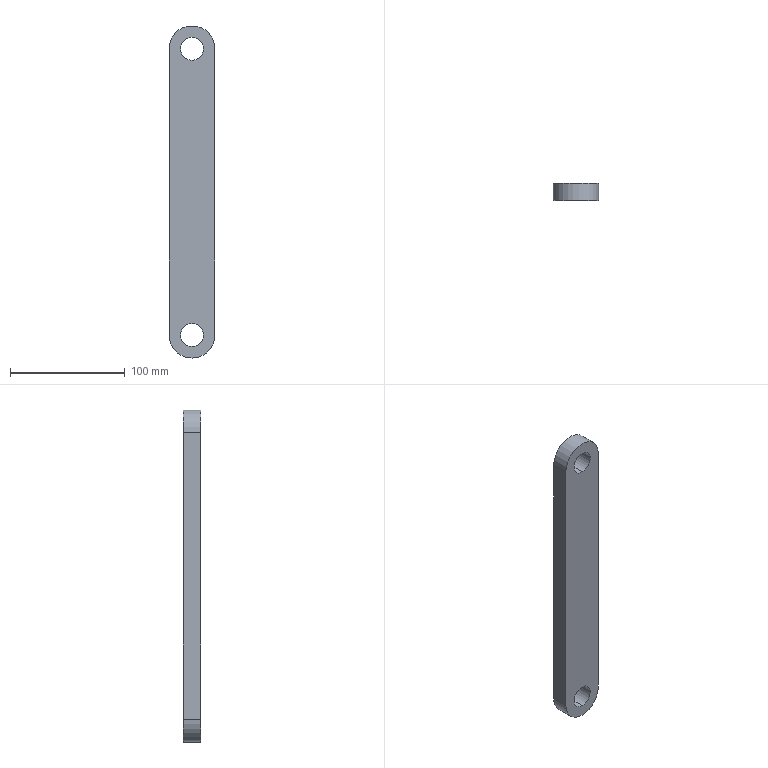Part | SolidWorks | features Extrusion 1 | 1 solid | 11 faces | box 40 x 15 x 290 mm | volume 159425 mm3 | cylinder 7 | plane 4 | commonest cylinder face diameters 20 x4 40 x3
STEP:
#1=CARTESIAN_POINT('',(0.,15.,-10.));
#2=VERTEX_POINT('',#1);
#3=CARTESIAN_POINT('',(0.,15.,10.));
#4=VERTEX_POINT('',#3);
#5=CARTESIAN_POINT('',(0.,15.,0.));
#6=DIRECTION('',(0.,1.,0.));
#7=DIRECTION('',(0.,0.,1.));
#8=AXIS2_PLACEMENT_3D('',#5,#6,#7);
#9=CIRCLE('',#8,10.);
#10=EDGE_CURVE('',#2,#4,#9,.T.);
#11=ORIENTED_EDGE('',*,*,#10,.T.);
#12=CARTESIAN_POINT('',(0.,0.,10.));
#13=VERTEX_POINT('',#12);
#14=CARTESIAN_POINT('',(0.,15.,10.));
#15=DIRECTION('',(0.,-1.,0.));
#16=VECTOR('',#15,1000.);
#17=LINE('',#14,#16);
#18=EDGE_CURVE('',#4,#13,#17,.T.);
#19=ORIENTED_EDGE('',*,*,#18,.T.);
#20=CARTESIAN_POINT('',(0.,0.,-10.));
#21=VERTEX_POINT('',#20);
#22=CARTESIAN_POINT('',(0.,0.,0.));
#23=DIRECTION('',(0.,1.,0.));
#24=DIRECTION('',(0.,0.,1.));
#25=AXIS2_PLACEMENT_3D('',#22,#23,#24);
#26=CIRCLE('',#25,10.);
#27=EDGE_CURVE('',#21,#13,#26,.T.);
#28=ORIENTED_EDGE('',*,*,#27,.F.);
#29=CARTESIAN_POINT('',(0.,15.,-10.));
#30=DIRECTION('',(0.,-1.,0.));
#31=VECTOR('',#30,1000.);
#32=LINE('',#29,#31);
#33=EDGE_CURVE('',#2,#21,#32,.T.);
#34=ORIENTED_EDGE('',*,*,#33,.F.);
#35=EDGE_LOOP('',(#11,#19,#28,#34));
#36=FACE_OUTER_BOUND('',#35,.T.);
#37=CARTESIAN_POINT('',(0.,15.,0.));
#38=DIRECTION('',(0.,-1.,0.));
#39=DIRECTION('',(0.,0.,-1.));
#40=AXIS2_PLACEMENT_3D('',#37,#38,#39);
#41=CYLINDRICAL_SURFACE('',#40,10.);
#42=ADVANCED_FACE('',(#36),#41,.F.);
#43=CARTESIAN_POINT('',(0.,15.,-260.));
#44=VERTEX_POINT('',#43);
#45=CARTESIAN_POINT('',(0.,15.,-240.));
#46=VERTEX_POINT('',#45);
#47=CARTESIAN_POINT('',(0.,15.,-250.));
#48=DIRECTION('',(0.,1.,0.));
#49=DIRECTION('',(0.,0.,1.));
#50=AXIS2_PLACEMENT_3D('',#47,#48,#49);
#51=CIRCLE('',#50,10.);
#52=EDGE_CURVE('',#44,#46,#51,.T.);
#53=ORIENTED_EDGE('',*,*,#52,.T.);
#54=CARTESIAN_POINT('',(0.,0.,-240.));
#55=VERTEX_POINT('',#54);
#56=CARTESIAN_POINT('',(0.,15.,-240.));
#57=DIRECTION('',(0.,-1.,0.));
#58=VECTOR('',#57,1000.);
#59=LINE('',#56,#58);
#60=EDGE_CURVE('',#46,#55,#59,.T.);
#61=ORIENTED_EDGE('',*,*,#60,.T.);
#62=CARTESIAN_POINT('',(0.,0.,-260.));
#63=VERTEX_POINT('',#62);
#64=CARTESIAN_POINT('',(0.,0.,-250.));
#65=DIRECTION('',(0.,1.,0.));
#66=DIRECTION('',(0.,0.,1.));
#67=AXIS2_PLACEMENT_3D('',#64,#65,#66);
#68=CIRCLE('',#67,10.);
#69=EDGE_CURVE('',#63,#55,#68,.T.);
#70=ORIENTED_EDGE('',*,*,#69,.F.);
#71=CARTESIAN_POINT('',(0.,15.,-260.));
#72=DIRECTION('',(0.,-1.,0.));
#73=VECTOR('',#72,1000.);
#74=LINE('',#71,#73);
#75=EDGE_CURVE('',#44,#63,#74,.T.);
#76=ORIENTED_EDGE('',*,*,#75,.F.);
#77=EDGE_LOOP('',(#53,#61,#70,#76));
#78=FACE_OUTER_BOUND('',#77,.T.);
#79=CARTESIAN_POINT('',(0.,15.,-250.));
#80=DIRECTION('',(0.,-1.,0.));
#81=DIRECTION('',(0.,0.,-1.));
#82=AXIS2_PLACEMENT_3D('',#79,#80,#81);
#83=CYLINDRICAL_SURFACE('',#82,10.);
#84=ADVANCED_FACE('',(#78),#83,.F.);
#85=CARTESIAN_POINT('',(0.,15.,-270.));
#86=VERTEX_POINT('',#85);
#87=CARTESIAN_POINT('',(-20.,15.,-250.));
#88=VERTEX_POINT('',#87);
#89=CARTESIAN_POINT('',(0.,15.,-250.));
#90=DIRECTION('',(0.,1.,0.));
#91=DIRECTION('',(0.,0.,1.));
#92=AXIS2_PLACEMENT_3D('',#89,#90,#91);
#93=CIRCLE('',#92,20.);
#94=EDGE_CURVE('',#86,#88,#93,.T.);
#95=ORIENTED_EDGE('',*,*,#94,.F.);
#96=CARTESIAN_POINT('',(0.,0.,-270.));
#97=VERTEX_POINT('',#96);
#98=CARTESIAN_POINT('',(0.,15.,-270.));
#99=DIRECTION('',(0.,-1.,0.));
#100=VECTOR('',#99,1000.);
#101=LINE('',#98,#100);
#102=EDGE_CURVE('',#86,#97,#101,.T.);
#103=ORIENTED_EDGE('',*,*,#102,.T.);
#104=CARTESIAN_POINT('',(-20.,0.,-250.));
#105=VERTEX_POINT('',#104);
#106=CARTESIAN_POINT('',(0.,0.,-250.));
#107=DIRECTION('',(0.,1.,0.));
#108=DIRECTION('',(0.,0.,1.));
#109=AXIS2_PLACEMENT_3D('',#106,#107,#108);
#110=CIRCLE('',#109,20.);
#111=EDGE_CURVE('',#97,#105,#110,.T.);
#112=ORIENTED_EDGE('',*,*,#111,.T.);
#113=CARTESIAN_POINT('',(-20.,15.,-250.));
#114=DIRECTION('',(0.,-1.,0.));
#115=VECTOR('',#114,1000.);
#116=LINE('',#113,#115);
#117=EDGE_CURVE('',#88,#105,#116,.T.);
#118=ORIENTED_EDGE('',*,*,#117,.F.);
#119=EDGE_LOOP('',(#95,#103,#112,#118));
#120=FACE_OUTER_BOUND('',#119,.T.);
#121=CARTESIAN_POINT('',(0.,15.,-250.));
#122=DIRECTION('',(0.,-1.,0.));
#123=DIRECTION('',(0.,0.,-1.));
#124=AXIS2_PLACEMENT_3D('',#121,#122,#123);
#125=CYLINDRICAL_SURFACE('',#124,20.);
#126=ADVANCED_FACE('',(#120),#125,.T.);
#127=ORIENTED_EDGE('',*,*,#52,.F.);
#128=CARTESIAN_POINT('',(0.,15.,-250.));
#129=DIRECTION('',(0.,1.,0.));
#130=DIRECTION('',(0.,0.,1.));
#131=AXIS2_PLACEMENT_3D('',#128,#129,#130);
#132=CIRCLE('',#131,10.);
#133=EDGE_CURVE('',#46,#44,#132,.T.);
#134=ORIENTED_EDGE('',*,*,#133,.F.);
#135=EDGE_LOOP('',(#127,#134));
#136=FACE_BOUND('',#135,.T.);
#137=CARTESIAN_POINT('',(-20.,15.,0.));
#138=VERTEX_POINT('',#137);
#139=CARTESIAN_POINT('',(20.,15.,0.));
#140=VERTEX_POINT('',#139);
#141=CARTESIAN_POINT('',(0.,15.,0.));
#142=DIRECTION('',(0.,1.,0.));
#143=DIRECTION('',(0.,0.,1.));
#144=AXIS2_PLACEMENT_3D('',#141,#142,#143);
#145=CIRCLE('',#144,20.);
#146=EDGE_CURVE('',#138,#140,#145,.T.);
#147=ORIENTED_EDGE('',*,*,#146,.T.);
#148=CARTESIAN_POINT('',(20.,15.,-250.));
#149=VERTEX_POINT('',#148);
#150=CARTESIAN_POINT('',(20.,15.,0.));
#151=DIRECTION('',(0.,0.,-1.));
#152=VECTOR('',#151,1000.);
#153=LINE('',#150,#152);
#154=EDGE_CURVE('',#140,#149,#153,.T.);
#155=ORIENTED_EDGE('',*,*,#154,.T.);
#156=CARTESIAN_POINT('',(0.,15.,-250.));
#157=DIRECTION('',(0.,1.,0.));
#158=DIRECTION('',(0.,0.,1.));
#159=AXIS2_PLACEMENT_3D('',#156,#157,#158);
#160=CIRCLE('',#159,20.);
#161=EDGE_CURVE('',#149,#86,#160,.T.);
#162=ORIENTED_EDGE('',*,*,#161,.T.);
#163=ORIENTED_EDGE('',*,*,#94,.T.);
#164=CARTESIAN_POINT('',(-20.,15.,0.));
#165=DIRECTION('',(0.,0.,1.));
#166=VECTOR('',#165,1000.);
#167=LINE('',#164,#166);
#168=EDGE_CURVE('',#88,#138,#167,.T.);
#169=ORIENTED_EDGE('',*,*,#168,.T.);
#170=EDGE_LOOP('',(#147,#155,#162,#163,#169));
#171=FACE_OUTER_BOUND('',#170,.T.);
#172=ORIENTED_EDGE('',*,*,#10,.F.);
#173=CARTESIAN_POINT('',(0.,15.,0.));
#174=DIRECTION('',(0.,1.,0.));
#175=DIRECTION('',(0.,0.,1.));
#176=AXIS2_PLACEMENT_3D('',#173,#174,#175);
#177=CIRCLE('',#176,10.);
#178=EDGE_CURVE('',#4,#2,#177,.T.);
#179=ORIENTED_EDGE('',*,*,#178,.F.);
#180=EDGE_LOOP('',(#172,#179));
#181=FACE_BOUND('',#180,.T.);
#182=CARTESIAN_POINT('',(0.,15.,0.));
#183=DIRECTION('',(0.,1.,0.));
#184=DIRECTION('',(0.,0.,1.));
#185=AXIS2_PLACEMENT_3D('',#182,#183,#184);
#186=PLANE('',#185);
#187=ADVANCED_FACE('',(#136,#171,#181),#186,.T.);
#188=CARTESIAN_POINT('',(-20.,0.,0.));
#189=VERTEX_POINT('',#188);
#190=CARTESIAN_POINT('',(20.,0.,0.));
#191=VERTEX_POINT('',#190);
#192=CARTESIAN_POINT('',(0.,0.,0.));
#193=DIRECTION('',(0.,1.,0.));
#194=DIRECTION('',(0.,0.,1.));
#195=AXIS2_PLACEMENT_3D('',#192,#193,#194);
#196=CIRCLE('',#195,20.);
#197=EDGE_CURVE('',#189,#191,#196,.T.);
#198=ORIENTED_EDGE('',*,*,#197,.F.);
#199=CARTESIAN_POINT('',(-20.,0.,0.));
#200=DIRECTION('',(0.,0.,1.));
#201=VECTOR('',#200,1000.);
#202=LINE('',#199,#201);
#203=EDGE_CURVE('',#105,#189,#202,.T.);
#204=ORIENTED_EDGE('',*,*,#203,.F.);
#205=ORIENTED_EDGE('',*,*,#111,.F.);
#206=CARTESIAN_POINT('',(20.,0.,-250.));
#207=VERTEX_POINT('',#206);
#208=CARTESIAN_POINT('',(0.,0.,-250.));
#209=DIRECTION('',(0.,1.,0.));
#210=DIRECTION('',(0.,0.,1.));
#211=AXIS2_PLACEMENT_3D('',#208,#209,#210);
#212=CIRCLE('',#211,20.);
#213=EDGE_CURVE('',#207,#97,#212,.T.);
#214=ORIENTED_EDGE('',*,*,#213,.F.);
#215=CARTESIAN_POINT('',(20.,0.,0.));
#216=DIRECTION('',(0.,0.,-1.));
#217=VECTOR('',#216,1000.);
#218=LINE('',#215,#217);
#219=EDGE_CURVE('',#191,#207,#218,.T.);
#220=ORIENTED_EDGE('',*,*,#219,.F.);
#221=EDGE_LOOP('',(#198,#204,#205,#214,#220));
#222=FACE_OUTER_BOUND('',#221,.T.);
#223=ORIENTED_EDGE('',*,*,#69,.T.);
#224=CARTESIAN_POINT('',(0.,0.,-250.));
#225=DIRECTION('',(0.,1.,0.));
#226=DIRECTION('',(0.,0.,1.));
#227=AXIS2_PLACEMENT_3D('',#224,#225,#226);
#228=CIRCLE('',#227,10.);
#229=EDGE_CURVE('',#55,#63,#228,.T.);
#230=ORIENTED_EDGE('',*,*,#229,.T.);
#231=EDGE_LOOP('',(#223,#230));
#232=FACE_BOUND('',#231,.T.);
#233=ORIENTED_EDGE('',*,*,#27,.T.);
#234=CARTESIAN_POINT('',(0.,0.,0.));
#235=DIRECTION('',(0.,1.,0.));
#236=DIRECTION('',(0.,0.,1.));
#237=AXIS2_PLACEMENT_3D('',#234,#235,#236);
#238=CIRCLE('',#237,10.);
#239=EDGE_CURVE('',#13,#21,#238,.T.);
#240=ORIENTED_EDGE('',*,*,#239,.T.);
#241=EDGE_LOOP('',(#233,#240));
#242=FACE_BOUND('',#241,.T.);
#243=CARTESIAN_POINT('',(0.,0.,0.));
#244=DIRECTION('',(0.,1.,0.));
#245=DIRECTION('',(0.,0.,1.));
#246=AXIS2_PLACEMENT_3D('',#243,#244,#245);
#247=PLANE('',#246);
#248=ADVANCED_FACE('',(#222,#232,#242),#247,.F.);
#249=ORIENTED_EDGE('',*,*,#197,.T.);
#250=CARTESIAN_POINT('',(20.,15.,0.));
#251=DIRECTION('',(0.,-1.,0.));
#252=VECTOR('',#251,1000.);
#253=LINE('',#250,#252);
#254=EDGE_CURVE('',#140,#191,#253,.T.);
#255=ORIENTED_EDGE('',*,*,#254,.F.);
#256=ORIENTED_EDGE('',*,*,#146,.F.);
#257=CARTESIAN_POINT('',(-20.,15.,0.));
#258=DIRECTION('',(0.,-1.,0.));
#259=VECTOR('',#258,1000.);
#260=LINE('',#257,#259);
#261=EDGE_CURVE('',#138,#189,#260,.T.);
#262=ORIENTED_EDGE('',*,*,#261,.T.);
#263=EDGE_LOOP('',(#249,#255,#256,#262));
#264=FACE_OUTER_BOUND('',#263,.T.);
#265=CARTESIAN_POINT('',(0.,15.,0.));
#266=DIRECTION('',(0.,-1.,0.));
#267=DIRECTION('',(0.,0.,-1.));
#268=AXIS2_PLACEMENT_3D('',#265,#266,#267);
#269=CYLINDRICAL_SURFACE('',#268,20.);
#270=ADVANCED_FACE('',(#264),#269,.T.);
#271=ORIENTED_EDGE('',*,*,#219,.T.);
#272=CARTESIAN_POINT('',(20.,15.,-250.));
#273=DIRECTION('',(0.,-1.,0.));
#274=VECTOR('',#273,1000.);
#275=LINE('',#272,#274);
#276=EDGE_CURVE('',#149,#207,#275,.T.);
#277=ORIENTED_EDGE('',*,*,#276,.F.);
#278=ORIENTED_EDGE('',*,*,#154,.F.);
#279=ORIENTED_EDGE('',*,*,#254,.T.);
#280=EDGE_LOOP('',(#271,#277,#278,#279));
#281=FACE_OUTER_BOUND('',#280,.T.);
#282=CARTESIAN_POINT('',(20.,15.,0.));
#283=DIRECTION('',(-1.,0.,0.));
#284=DIRECTION('',(0.,0.,1.));
#285=AXIS2_PLACEMENT_3D('',#282,#283,#284);
#286=PLANE('',#285);
#287=ADVANCED_FACE('',(#281),#286,.F.);
#288=ORIENTED_EDGE('',*,*,#102,.F.);
#289=ORIENTED_EDGE('',*,*,#161,.F.);
#290=ORIENTED_EDGE('',*,*,#276,.T.);
#291=ORIENTED_EDGE('',*,*,#213,.T.);
#292=EDGE_LOOP('',(#288,#289,#290,#291));
#293=FACE_OUTER_BOUND('',#292,.T.);
#294=CARTESIAN_POINT('',(0.,15.,-250.));
#295=DIRECTION('',(0.,-1.,0.));
#296=DIRECTION('',(0.,0.,-1.));
#297=AXIS2_PLACEMENT_3D('',#294,#295,#296);
#298=CYLINDRICAL_SURFACE('',#297,20.);
#299=ADVANCED_FACE('',(#293),#298,.T.);
#300=ORIENTED_EDGE('',*,*,#203,.T.);
#301=ORIENTED_EDGE('',*,*,#261,.F.);
#302=ORIENTED_EDGE('',*,*,#168,.F.);
#303=ORIENTED_EDGE('',*,*,#117,.T.);
#304=EDGE_LOOP('',(#300,#301,#302,#303));
#305=FACE_OUTER_BOUND('',#304,.T.);
#306=CARTESIAN_POINT('',(-20.,15.,0.));
#307=DIRECTION('',(1.,0.,0.));
#308=DIRECTION('',(0.,0.,-1.));
#309=AXIS2_PLACEMENT_3D('',#306,#307,#308);
#310=PLANE('',#309);
#311=ADVANCED_FACE('',(#305),#310,.F.);
#312=ORIENTED_EDGE('',*,*,#60,.F.);
#313=ORIENTED_EDGE('',*,*,#133,.T.);
#314=ORIENTED_EDGE('',*,*,#75,.T.);
#315=ORIENTED_EDGE('',*,*,#229,.F.);
#316=EDGE_LOOP('',(#312,#313,#314,#315));
#317=FACE_OUTER_BOUND('',#316,.T.);
#318=CARTESIAN_POINT('',(0.,15.,-250.));
#319=DIRECTION('',(0.,-1.,0.));
#320=DIRECTION('',(0.,0.,-1.));
#321=AXIS2_PLACEMENT_3D('',#318,#319,#320);
#322=CYLINDRICAL_SURFACE('',#321,10.);
#323=ADVANCED_FACE('',(#317),#322,.F.);
#324=ORIENTED_EDGE('',*,*,#18,.F.);
#325=ORIENTED_EDGE('',*,*,#178,.T.);
#326=ORIENTED_EDGE('',*,*,#33,.T.);
#327=ORIENTED_EDGE('',*,*,#239,.F.);
#328=EDGE_LOOP('',(#324,#325,#326,#327));
#329=FACE_OUTER_BOUND('',#328,.T.);
#330=CARTESIAN_POINT('',(0.,15.,0.));
#331=DIRECTION('',(0.,-1.,0.));
#332=DIRECTION('',(0.,0.,-1.));
#333=AXIS2_PLACEMENT_3D('',#330,#331,#332);
#334=CYLINDRICAL_SURFACE('',#333,10.);
#335=ADVANCED_FACE('',(#329),#334,.F.);
#336=CLOSED_SHELL('',(#42,#84,#126,#187,#248,#270,#287,#299,#311,#323,#335));
#337=MANIFOLD_SOLID_BREP('',#336);
#338=CARTESIAN_POINT('',(0.,0.,0.));
#339=DIRECTION('',(0.,0.,1.));
#340=DIRECTION('',(1.,0.,0.));
#341=AXIS2_PLACEMENT_3D('',#338,#339,#340);
#342=(LENGTH_UNIT()NAMED_UNIT(*)SI_UNIT(.MILLI.,.METRE.));
#343=UNCERTAINTY_MEASURE_WITH_UNIT(LENGTH_MEASURE(0.00001),#342,'','');
#344=(NAMED_UNIT(*)PLANE_ANGLE_UNIT()SI_UNIT($,.RADIAN.));
#345=(NAMED_UNIT(*)SI_UNIT($,.STERADIAN.)SOLID_ANGLE_UNIT());
#346=(GEOMETRIC_REPRESENTATION_CONTEXT(3)GLOBAL_UNCERTAINTY_ASSIGNED_CONTEXT((#343))GLOBAL_UNIT_ASSIGNED_CONTEXT((#342,#344,#345))REPRESENTATION_CONTEXT('',''));
#347=ADVANCED_BREP_SHAPE_REPRESENTATION('',(#337,#341),#346);